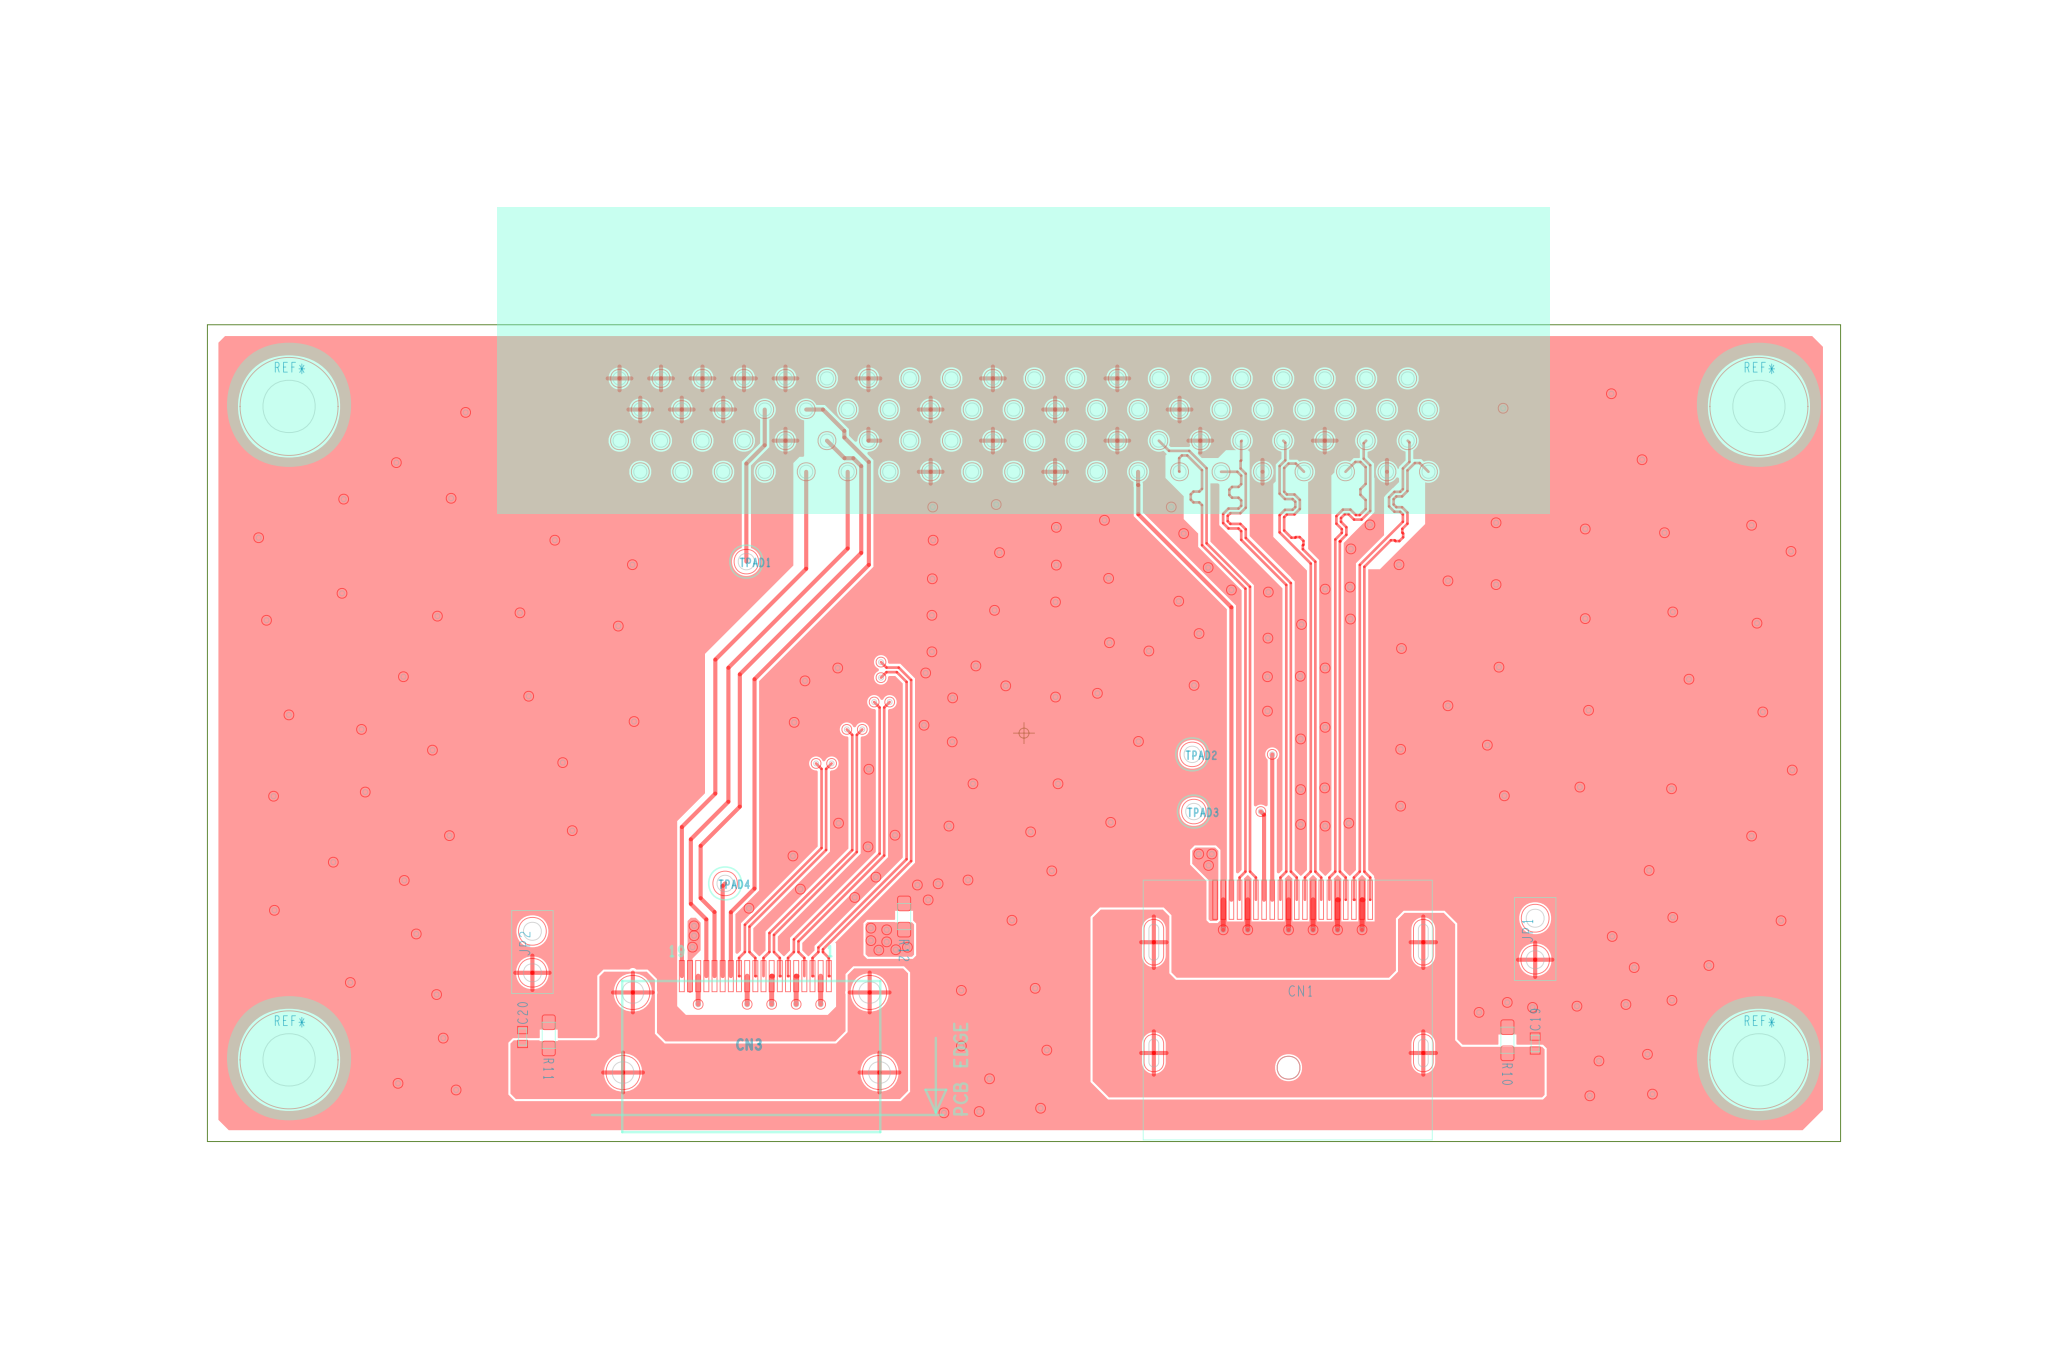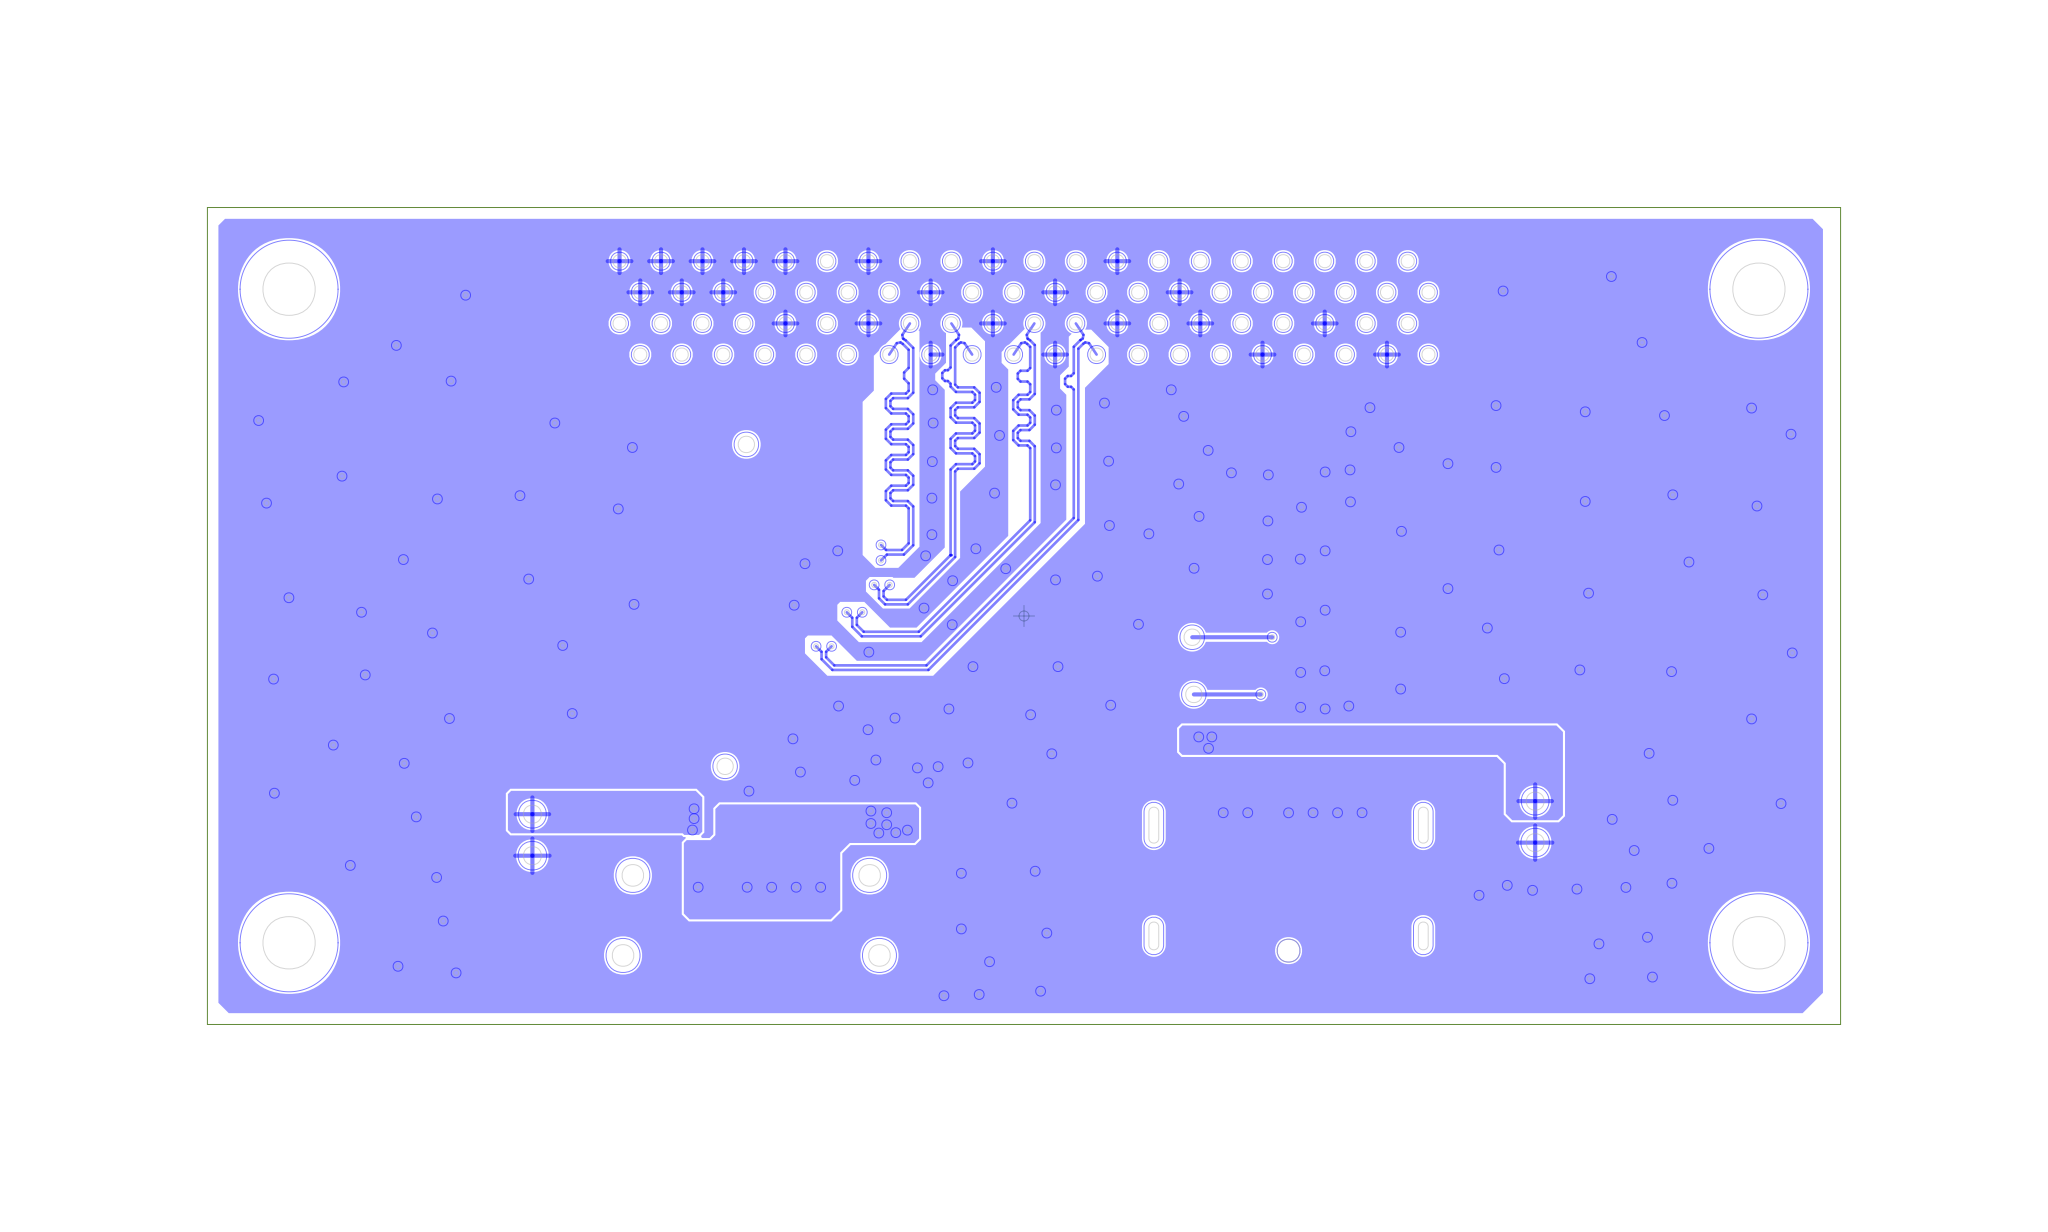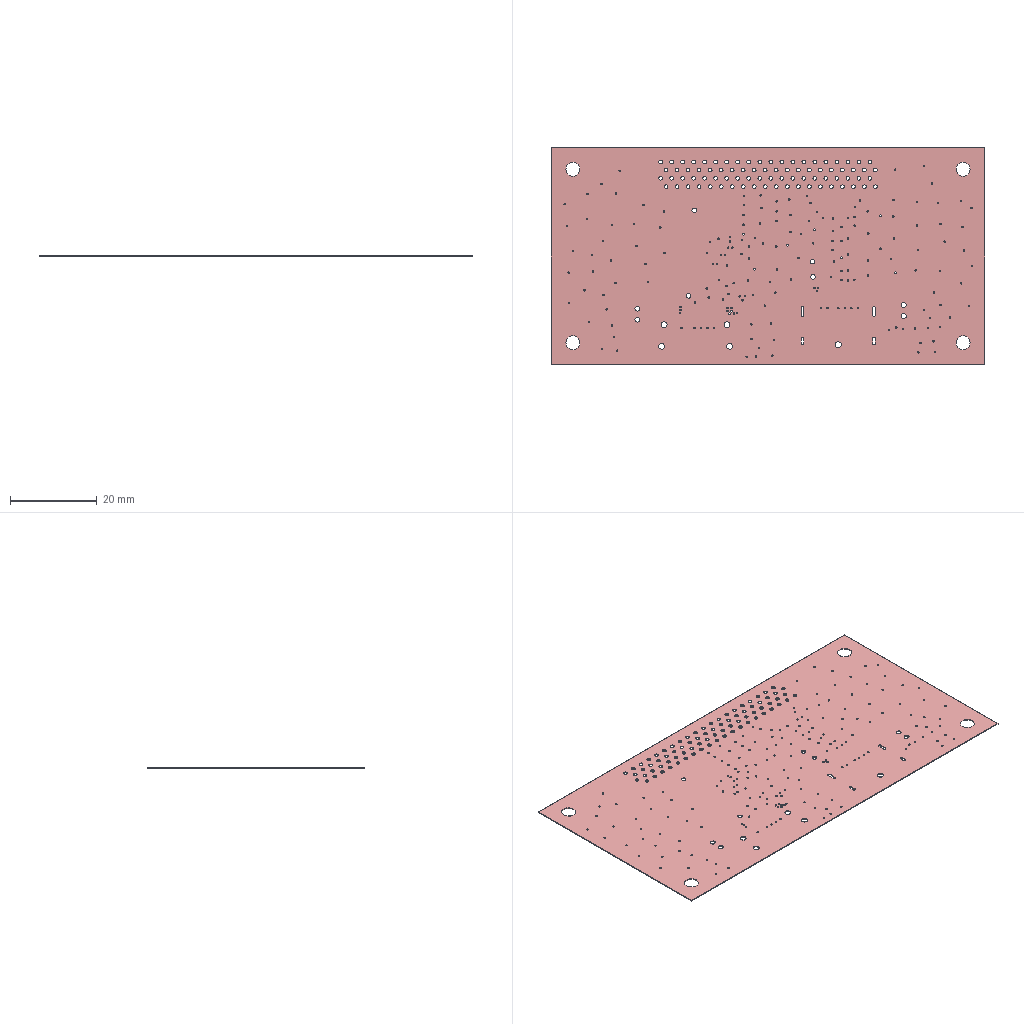Circuit board layout | Cadence Allegro | box 100 x 50 x 0.2 mm
Layer stack:
# Cadence Allegro layer stack of  (unit mm; from the constraint file cross-section; dielectric type: 0 not recorded (Allegro does not mark core vs prepreg), 3 surface material)
index,name,kind,layer,copper_thickness_mm,dielectric_type,dielectric_thickness_mm,dielectric_material,dielectric_constant
0,Top Surface,other,,,,,,
1,TOP,copper,TOP,0.0305,,,,
2,Dielectric1,dielectric,,,0,0.2032,FR-4,4.5
3,BOTTOM,copper,BOTTOM,0.0305,,,,
4,Bottom Surface,other,,,,,,
# drill layer pairs: low layer,high layer
drill_pair,TOP,BOTTOM
Part placement:
REFDES,COMP_VALUE,SYM_NAME,SYM_X,SYM_Y,SYM_ROTATE,SYM_MIRROR
C19,1uF,1005,1232.283,-748.031,90.000,NO
C20,1uF,1005,-1208.657,-732.283,90.000,NO
CN1,DP1RD20JQ1R400,DP1RD20JQ1R400,637.795,-503.937,0.000,NO
CN2,TX25-80P-LT-N1E,TX25-80P-LT-N1E,0.000,629.921,0.000,NO
CN3,10029449-001RLF,CON_HDMI_19F_20_SM_RA,-657.480,-779.528,0.000,NO
JP1,XG8T-0231,HDR1X2-2_54,1232.283,-496.063,90.000,NO
JP2,XG8T-0231,HDR1X2-2_54,-1185.039,-527.559,90.000,NO
R10,1M,1608,1165.354,-740.157,270.000,NO
R11,1M,1608,-1145.669,-728.346,270.000,NO
R12,0,1608,-289.000,-442.000,270.000,NO
TPAD1,M1.0,TH_TC15-C10,-669.291,413.386,0.000,NO
TPAD2,M1.0,TH_TC15-C10,405.512,-51.181,0.000,NO
TPAD3,M1.0,TH_TC15-C10,409.449,-188.976,0.000,NO
TPAD4,M1.0,TH_TC15-C10,-720.472,-362.205,0.000,NO
Pad and via stacks:
# Allegro (Cadence) via spans and padstacks; design units: ("mils" 3 1000)
# via spans: padstack,start_layer,end_layer,net_example,count
VIA,ETCH/TOP,ETCH/BOTTOM,DGND,191
# Allegro padstack definitions: name,start_layer,end_layer,drill,plating,holeType,type
R045-060-02,"ETCH/TOP","ETCH/TOP",0.0,"PLATED","none","smd"
REC02802400,"ETCH/TOP","ETCH/TOP",0.0,"PLATED","none","smd"
R012X075S,"ETCH/TOP","ETCH/TOP",0.0,"PLATED","none","smd"
CRC1608-PAD,"ETCH/TOP","ETCH/TOP",0.0,"PLATED","none","smd"
C150TC100-01,"ETCH/TOP","ETCH/BOTTOM",125.984,"PLATED","circle_drill","through"
CIR1400,"ETCH/TOP","ETCH/BOTTOM",55.118,"NON_PLATED","circle_drill","through"
OBL17000600,"ETCH/TOP","ETCH/BOTTOM",23.622,"NON_PLATED","oval slot","through"
OBL22000600,"ETCH/TOP","ETCH/BOTTOM",23.622,"NON_PLATED","oval slot","through"
Y8,"ETCH/TOP","ETCH/BOTTOM",31.496,"PLATED","circle_drill","through"
C082-052T_TOL2_2,"ETCH/TOP","ETCH/BOTTOM",52.0,"PLATED","circle_drill","through"
MPS1100CA,"ETCH/TOP","ETCH/BOTTOM",43.307,"PLATED","circle_drill","through"
MP1100CA,"ETCH/TOP","ETCH/BOTTOM",43.307,"PLATED","circle_drill","through"
TC15-C10,"ETCH/TOP","ETCH/BOTTOM",39.37,"PLATED","circle_drill","through"
VIA,"ETCH/TOP","ETCH/BOTTOM",11.811,"PLATED","circle_drill","through"
Design rules, without the lines most boards share, first 16 of 33 lines:
# Cadence Allegro design rules of  (from the Constraint Manager export constraints.dcfx, design unit mil; typed fields in mm)
# columns: name | kind | enabled | priority | scope1 | scope2 | descriptor | typed fields (field=value)
# Allegro precedence (priority 1 wins): 1 Region class-to-class, 2 Region class, 3 Region, 4 class-to-class, 5 DiffPair/Bus/NetGroup override, 6 NetClass, 7 constraint set (CSet) default
# per-layer values are written LAYER=value in the descriptor and LAYER:mm in the typed field; a maximum of 0 means no limit set
# --- net classes (and buses / net groups) ---
DDP | NetClass | enabled | 6 | DDP_AU, DDP_0, DDP_1, DDP_2, DDP_3 | All | Net Class (ElectricalCSet=CF) (members: 5 DiffPair) | electricalcset=CF
HDMI | NetClass | enabled | 6 | HDMI_CKIN0, HDMI_IN0, HDMI_IN1, HDMI_IN2 | All | Net Class (ElectricalCSet=CF) (members: 4 DiffPair) | electricalcset=CF
# --- track widths, neck and differential-pair gap (physical constraint sets) ---
DEFAULT | PhysicalCSet | enabled | 7 | Design default | All | Physical Constraint (Min Line Width=10mil) (Max Line Width=20mil) (Min Neck Width=10mil) (Max Neck Length=10mil) (DiffPair Primary Gap=0mil) (DiffPair Neck Gap=0mil) (DiffPair Min Space=0mil) (DiffPair Coupled +Tol=0mil) (DiffPair Coupled -Tol=0mil) (Min BB Via Stagger=5mil) (Max BB Via Stagger=0mil) (T-junctions=ANYWHERE) (Pad-pad direct connect=ALL_ALLOWED) (Allowed vias=VIA) | min_line_width=0.254 min_neck_width=0.254 min_bvia_stagger=0.127 max_bvia_stagger=0 ts_allowed=ANYWHERE diffp_primary_gap=0 diffp_neck_gap=0 max_line_width=0.508 maximum_neck_length=0.254 pad_pad_direct_connect=ALL_ALLOWED allow_on_etch_subclass=TRUE diffp_coupled_plus=0 diffp_coupled_minus=0 diffp_min_space=0 vias=VIA
# --- clearances: line / pad / via / shape / hole (spacing constraint sets) ---
DEFAULT | SpacingCSet | enabled | 7 | Design default | All | Clearance Constraint (Line-Line=6mil) (Line-SMD Pad=6mil) (Line-Thru Pin=6mil) (Line-Via=6mil) (Line-Shape=6mil) (SMD Pad-SMD Pad=5mil) (Thru Pin-Thru Pin=5mil) (Thru Pin-SMD Pad=5mil) (SMD Pad-Via=5mil) (Thru Pin-Via=5mil) (Via-Via=5mil) (Shape-SMD Pad=5mil) (Shape-Thru Pin=5mil) (Shape-Via=5mil) (Shape-Shape=5mil) (Hole-Hole=8mil) (Hole-Line=6mil) (Hole-Shape=8mil) (BB Via-BB Via=5mil) (uVia-uVia=5mil) | thrupin_to_thrupin_spacing=0.127 thrupin_to_smdpin_spacing=0.127 thrupin_to_thruvia_spacing=0.127 line_to_thrupin_spacing=0.1524 thrupin_to_shape_spacing=0.127 smdpin_to_smdpin_spacing=0.127 smdpin_to_thruvia_spacing=0.127 line_to_smdpin_spacing=0.1524 shape_to_smdpin_spacing=0.127 thruvia_to_thruvia_spacing=0.127 line_to_thruvia_spacing=0.1524 shape_to_thruvia_spacing=0.127 line_to_line_spacing=0.1524 line_to_shape_spacing=0.1524 shape_to_shape_spacing=0.127 bbv_to_bbv_spacing=0.127 bbv_to_thrupin_spacing=0.127 bbv_to_smdpin_spacing=0.127 bbv_to_thruvia_spacing=0.127 bbv_to_line_spacing=0.1524 bbv_to_shape_spacing=0.127 bbv_to_testpin_spacing=0.127 bbv_to_testvia_spacing=0.127 testpin_to_testpin_spacing=0.127 testpin_to_thrupin_spacing=0.127 smdpin_to_testpin_spacing=0.127 testpin_to_thruvia_spacing=0.127 testpin_to_testvia_spacing=0.127 line_to_testpin_spacing=0.1524 shape_to_testpin_spacing=0.127 testvia_to_testvia_spacing=0.127 testvia_to_thrupin_spacing=0.127 smdpin_to_testvia_spacing=0.127 testvia_to_thruvia_spacing=0.127 line_to_testvia_spacing=0.1524 shape_to_testvia_spacing=0.127 bondpad_to_bondpad_spacing=0.127 thrupin_to_bondpad_spacing=0.127 smdpin_to_bondpad_spacing=0.127 bondpad_to_thruvia_spacing=0.127 bondpad_to_line_spacing=0.1524 bondpad_to_shape_spacing=0.127 bondpad_to_bbv_spacing=0.127 bondpad_to_testpin_spacing=0.127 bondpad_to_testvia_spacing=0.127 min_bvia_gap=0.127 hole_to_pin_spacing=0.2032 hole_to_via_spacing=0.2032 hole_to_line_spacing=0.1524 hole_to_shape_spacing=0.2032 hole_to_hole_spacing=0.2032 mvia_to_mvia_spacing=0.127 mvia_to_thrupin_spacing=0.127 mvia_to_smdpin_spacing=0.127 mvia_to_thruvia_spacing=0.127 mvia_to_bbv_spacing=0.127 mvia_to_line_spacing=0.1524 mvia_to_shape_spacing=0.127 mvia_to_testpin_spacing=0.127 mvia_to_testvia_spacing=0.127 bondpad_to_mvia_spacing=0.127 bondpad_to_bondpad_diffp_spc=0.127
DEFAULT | SameNetSpacingCSet | disabled (SAME_NET=FALSE) | 7 | Design default | All | Same-Net Clearance (Line-Line=5mil) (Line-SMD Pad=5mil) (Line-Thru Pin=5mil) (Line-Via=5mil) (Line-Shape=5mil) (SMD Pad-SMD Pad=5mil) (Thru Pin-Thru Pin=5mil) (Thru Pin-SMD Pad=5mil) (SMD Pad-Via=5mil) (Thru Pin-Via=5mil) (Via-Via=5mil) (Shape-SMD Pad=5mil) (Shape-Thru Pin=5mil) (Shape-Via=5mil) (Shape-Shape=5mil) (Hole-Hole=8mil) (Hole-Line=8mil) (Hole-Shape=8mil) (BB Via-BB Via=5mil) (uVia-uVia=5mil) | sn_thrupin_to_thrupin_spacing=0.127 sn_thrupin_to_smdpin_spacing=0.127 sn_thrupin_to_thruvia_spacing=0.127 sn_line_to_thrupin_spacing=0.127 sn_thrupin_to_shape_spacing=0.127 sn_smdpin_to_smdpin_spacing=0.127 sn_smdpin_to_thruvia_spacing=0.127 sn_line_to_smdpin_spacing=0.127 sn_shape_to_smdpin_spacing=0.127 sn_thruvia_to_thruvia_spacing=0.127 sn_line_to_thruvia_spacing=0.127 sn_shape_to_thruvia_spacing=0.127 sn_line_to_line_spacing=0.127 sn_line_to_shape_spacing=0.127 sn_shape_to_shape_spacing=0.127 sn_bbv_to_bbv_spacing=0.127 sn_bbv_to_thrupin_spacing=0.127 sn_bbv_to_smdpin_spacing=0.127 sn_bbv_to_thruvia_spacing=0.127 sn_bbv_to_line_spacing=0.127 sn_bbv_to_shape_spacing=0.127 sn_bbv_to_testpin_spacing=0.127 sn_bbv_to_testvia_spacing=0.127 sn_testpin_to_testpin_spacing=0.127 sn_testpin_to_thrupin_spacing=0.127 sn_smdpin_to_testpin_spacing=0.127 sn_testpin_to_thruvia_spacing=0.127 sn_testpin_to_testvia_spacing=0.127 sn_line_to_testpin_spacing=0.127 sn_shape_to_testpin_spacing=0.127 sn_testvia_to_testvia_spacing=0.127 sn_testvia_to_thrupin_spacing=0.127 sn_smdpin_to_testvia_spacing=0.127 sn_testvia_to_thruvia_spacing=0.127 sn_line_to_testvia_spacing=0.127 sn_shape_to_testvia_spacing=0.127 sn_bondpad_to_bondpad_spacing=0.127 sn_thrupin_to_bondpad_spacing=0.127 sn_smdpin_to_bondpad_spacing=0.127 sn_bondpad_to_thruvia_spacing=0.127 sn_bondpad_to_line_spacing=0.127 sn_bondpad_to_shape_spacing=0.127 sn_bondpad_to_bbv_spacing=0.127 sn_bondpad_to_testpin_spacing=0.127 sn_bondpad_to_testvia_spacing=0.127 same_net=FALSE sn_hole_to_pin_spacing=0.2032 sn_hole_to_via_spacing=0.2032 sn_hole_to_line_spacing=0.2032 sn_hole_to_shape_spacing=0.2032 sn_hole_to_hole_spacing=0.2032 sn_mvia_to_mvia_spacing=0.127 sn_mvia_to_thrupin_spacing=0.127 sn_mvia_to_smdpin_spacing=0.127 sn_mvia_to_thruvia_spacing=0.127 sn_mvia_to_bbv_spacing=0.127 sn_mvia_to_line_spacing=0.127 sn_mvia_to_shape_spacing=0.127 sn_mvia_to_testpin_spacing=0.127 sn_mvia_to_testvia_spacing=0.127 sn_bondpad_to_mvia_spacing=0.127
# --- differential pairs (9) ---
DDP_AU | DiffPair | enabled | 5 | DDP_AUXN | DDP_AUXP | Differential Pair (Primary Gap=0mil) (Min Line Width=10mil) (Physical CSet=DEFAULT) | gap=0 width=0.254 electricalcset=CF
DDP_0 | DiffPair | enabled | 5 | DDP_0N | DDP_0P | Differential Pair (Primary Gap=0mil) (Min Line Width=10mil) (Physical CSet=DEFAULT) | gap=0 width=0.254 electricalcset=CF
DDP_1 | DiffPair | enabled | 5 | DDP_1N | DDP_1P | Differential Pair (Primary Gap=0mil) (Min Line Width=10mil) (Physical CSet=DEFAULT) | gap=0 width=0.254 electricalcset=CF